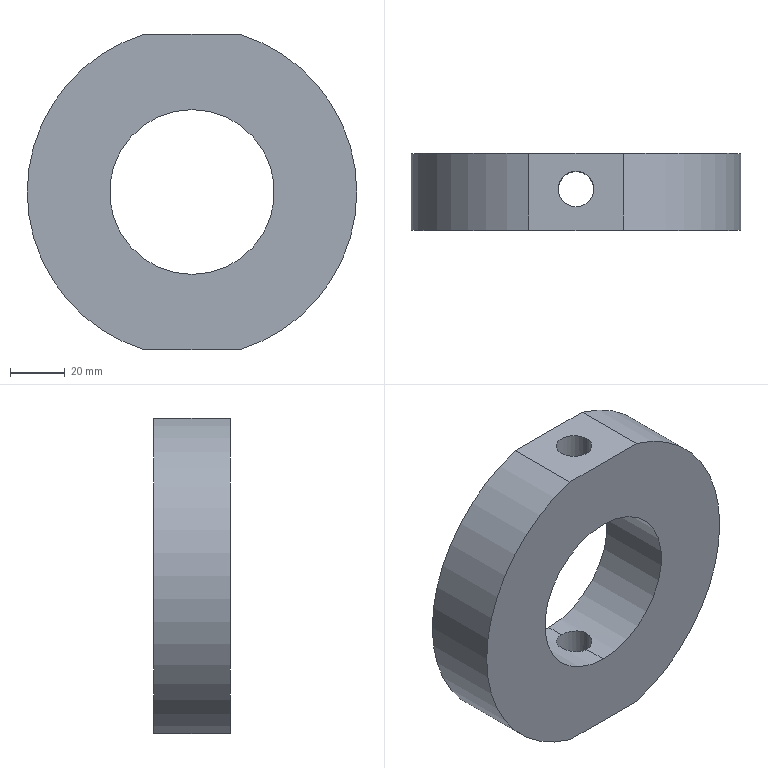Part | SolidWorks | features ICE 2, Extrusion 1 | 1 solid | 12 faces | box 120 x 28 x 115 mm | volume 226944 mm3 | cylinder 8 | plane 4 | commonest cylinder face diameters 13 x4 60 x2 120 x2
STEP:
#1=CARTESIAN_POINT('',(0.,-5.5,30.));
#2=VERTEX_POINT('',#1);
#3=CARTESIAN_POINT('',(-6.5,1.,29.287));
#4=VERTEX_POINT('',#3);
#5=CARTESIAN_POINT('',(0.,-5.5,30.));
#6=CARTESIAN_POINT('',(-0.4253,-5.5,30.));
#7=CARTESIAN_POINT('',(-0.8574,-5.457,29.991));
#8=CARTESIAN_POINT('',(-1.692,-5.29,29.955));
#9=CARTESIAN_POINT('',(-2.097,-5.167,29.929));
#10=CARTESIAN_POINT('',(-2.689,-4.922,29.88));
#11=CARTESIAN_POINT('',(-2.883,-4.829,29.862));
#12=CARTESIAN_POINT('',(-3.258,-4.628,29.823));
#13=CARTESIAN_POINT('',(-3.44,-4.519,29.803));
#14=CARTESIAN_POINT('',(-3.967,-4.167,29.739));
#15=CARTESIAN_POINT('',(-4.296,-3.896,29.692));
#16=CARTESIAN_POINT('',(-4.899,-3.293,29.599));
#17=CARTESIAN_POINT('',(-5.167,-2.966,29.553));
#18=CARTESIAN_POINT('',(-5.52,-2.439,29.488));
#19=CARTESIAN_POINT('',(-5.629,-2.257,29.467));
#20=CARTESIAN_POINT('',(-5.831,-1.88,29.428));
#21=CARTESIAN_POINT('',(-5.923,-1.686,29.41));
#22=CARTESIAN_POINT('',(-6.167,-1.097,29.36));
#23=CARTESIAN_POINT('',(-6.29,-0.692,29.333));
#24=CARTESIAN_POINT('',(-6.416,-0.06519,29.306));
#25=CARTESIAN_POINT('',(-6.448,0.1482,29.299));
#26=CARTESIAN_POINT('',(-6.49,0.5748,29.29));
#27=CARTESIAN_POINT('',(-6.5,0.7876,29.287));
#28=CARTESIAN_POINT('',(-6.5,1.,29.287));
#29=B_SPLINE_CURVE_WITH_KNOTS('',3,(#5,#6,#7,#8,#9,#10,#11,#12,#13,#14,#15,#16,#17,#18,#19,#20,#21,#22,#23,#24,#25,#26,#27,#28),.UNSPECIFIED.,.F.,.F.,(4,2,2,2,2,2,2,2,2,2,2,4),(0.01019,0.01147,0.01274,0.01338,0.01401,0.01529,0.01656,0.0172,0.01784,0.01911,0.01975,0.02038),.UNSPECIFIED.);
#30=EDGE_CURVE('',#2,#4,#29,.T.);
#31=ORIENTED_EDGE('',*,*,#30,.T.);
#32=CARTESIAN_POINT('',(-6.5,1.,57.5));
#33=VERTEX_POINT('',#32);
#34=CARTESIAN_POINT('',(-6.5,1.,-57.5));
#35=DIRECTION('',(0.,0.,1.));
#36=VECTOR('',#35,1000.);
#37=LINE('',#34,#36);
#38=EDGE_CURVE('',#4,#33,#37,.T.);
#39=ORIENTED_EDGE('',*,*,#38,.T.);
#40=CARTESIAN_POINT('',(6.5,1.,57.5));
#41=VERTEX_POINT('',#40);
#42=CARTESIAN_POINT('',(0.,1.,57.5));
#43=DIRECTION('',(0.,0.,1.));
#44=DIRECTION('',(1.,0.,0.));
#45=AXIS2_PLACEMENT_3D('',#42,#43,#44);
#46=CIRCLE('',#45,6.5);
#47=EDGE_CURVE('',#33,#41,#46,.T.);
#48=ORIENTED_EDGE('',*,*,#47,.T.);
#49=CARTESIAN_POINT('',(6.5,1.,29.287));
#50=VERTEX_POINT('',#49);
#51=CARTESIAN_POINT('',(6.5,1.,-57.5));
#52=DIRECTION('',(0.,0.,1.));
#53=VECTOR('',#52,1000.);
#54=LINE('',#51,#53);
#55=EDGE_CURVE('',#50,#41,#54,.T.);
#56=ORIENTED_EDGE('',*,*,#55,.F.);
#57=CARTESIAN_POINT('',(6.5,1.,29.287));
#58=CARTESIAN_POINT('',(6.5,0.569,29.287));
#59=CARTESIAN_POINT('',(6.458,0.1455,29.297));
#60=CARTESIAN_POINT('',(6.333,-0.479,29.324));
#61=CARTESIAN_POINT('',(6.281,-0.6854,29.335));
#62=CARTESIAN_POINT('',(6.157,-1.095,29.361));
#63=CARTESIAN_POINT('',(6.084,-1.298,29.377));
#64=CARTESIAN_POINT('',(5.839,-1.888,29.427));
#65=CARTESIAN_POINT('',(5.639,-2.26,29.466));
#66=CARTESIAN_POINT('',(5.167,-2.966,29.553));
#67=CARTESIAN_POINT('',(4.893,-3.299,29.6));
#68=CARTESIAN_POINT('',(4.295,-3.897,29.692));
#69=CARTESIAN_POINT('',(3.969,-4.166,29.738));
#70=CARTESIAN_POINT('',(3.258,-4.641,29.825));
#71=CARTESIAN_POINT('',(2.882,-4.842,29.864));
#72=CARTESIAN_POINT('',(2.295,-5.085,29.913));
#73=CARTESIAN_POINT('',(2.095,-5.157,29.927));
#74=CARTESIAN_POINT('',(1.688,-5.281,29.953));
#75=CARTESIAN_POINT('',(1.478,-5.333,29.964));
#76=CARTESIAN_POINT('',(0.8483,-5.459,29.991));
#77=CARTESIAN_POINT('',(0.4255,-5.5,30.));
#78=CARTESIAN_POINT('',(0.,-5.5,30.));
#79=B_SPLINE_CURVE_WITH_KNOTS('',3,(#57,#58,#59,#60,#61,#62,#63,#64,#65,#66,#67,#68,#69,#70,#71,#72,#73,#74,#75,#76,#77,#78),.UNSPECIFIED.,.F.,.F.,(4,2,2,2,2,2,2,2,2,2,4),(0.,0.001274,0.001911,0.002548,0.003823,0.005097,0.006371,0.007645,0.008282,0.00892,0.01019),.UNSPECIFIED.);
#80=EDGE_CURVE('',#50,#2,#79,.T.);
#81=ORIENTED_EDGE('',*,*,#80,.T.);
#82=EDGE_LOOP('',(#31,#39,#48,#56,#81));
#83=FACE_OUTER_BOUND('',#82,.T.);
#84=CARTESIAN_POINT('',(0.,1.,-57.5));
#85=DIRECTION('',(0.,0.,1.));
#86=DIRECTION('',(1.,0.,0.));
#87=AXIS2_PLACEMENT_3D('',#84,#85,#86);
#88=CYLINDRICAL_SURFACE('',#87,6.5);
#89=ADVANCED_FACE('',(#83),#88,.F.);
#90=CARTESIAN_POINT('',(-6.5,1.,-57.5));
#91=VERTEX_POINT('',#90);
#92=CARTESIAN_POINT('',(6.5,1.,-57.5));
#93=VERTEX_POINT('',#92);
#94=CARTESIAN_POINT('',(0.,1.,-57.5));
#95=DIRECTION('',(0.,0.,1.));
#96=DIRECTION('',(1.,0.,0.));
#97=AXIS2_PLACEMENT_3D('',#94,#95,#96);
#98=CIRCLE('',#97,6.5);
#99=EDGE_CURVE('',#91,#93,#98,.T.);
#100=ORIENTED_EDGE('',*,*,#99,.F.);
#101=CARTESIAN_POINT('',(-6.5,1.,-29.287));
#102=VERTEX_POINT('',#101);
#103=CARTESIAN_POINT('',(-6.5,1.,-57.5));
#104=DIRECTION('',(0.,0.,1.));
#105=VECTOR('',#104,1000.);
#106=LINE('',#103,#105);
#107=EDGE_CURVE('',#91,#102,#106,.T.);
#108=ORIENTED_EDGE('',*,*,#107,.T.);
#109=CARTESIAN_POINT('',(0.,-5.5,-30.));
#110=VERTEX_POINT('',#109);
#111=CARTESIAN_POINT('',(-6.5,1.,-29.287));
#112=CARTESIAN_POINT('',(-6.5,0.5747,-29.287));
#113=CARTESIAN_POINT('',(-6.457,0.1426,-29.297));
#114=CARTESIAN_POINT('',(-6.29,-0.6917,-29.333));
#115=CARTESIAN_POINT('',(-6.167,-1.097,-29.36));
#116=CARTESIAN_POINT('',(-5.922,-1.689,-29.41));
#117=CARTESIAN_POINT('',(-5.829,-1.883,-29.428));
#118=CARTESIAN_POINT('',(-5.628,-2.258,-29.467));
#119=CARTESIAN_POINT('',(-5.519,-2.44,-29.488));
#120=CARTESIAN_POINT('',(-5.167,-2.966,-29.553));
#121=CARTESIAN_POINT('',(-4.896,-3.296,-29.599));
#122=CARTESIAN_POINT('',(-4.293,-3.899,-29.693));
#123=CARTESIAN_POINT('',(-3.966,-4.167,-29.739));
#124=CARTESIAN_POINT('',(-3.439,-4.52,-29.803));
#125=CARTESIAN_POINT('',(-3.257,-4.629,-29.823));
#126=CARTESIAN_POINT('',(-2.88,-4.831,-29.862));
#127=CARTESIAN_POINT('',(-2.686,-4.923,-29.88));
#128=CARTESIAN_POINT('',(-2.097,-5.167,-29.929));
#129=CARTESIAN_POINT('',(-1.692,-5.29,-29.955));
#130=CARTESIAN_POINT('',(-1.065,-5.416,-29.982));
#131=CARTESIAN_POINT('',(-0.8518,-5.448,-29.989));
#132=CARTESIAN_POINT('',(-0.4252,-5.49,-29.998));
#133=CARTESIAN_POINT('',(-0.2124,-5.5,-30.));
#134=CARTESIAN_POINT('',(0.,-5.5,-30.));
#135=B_SPLINE_CURVE_WITH_KNOTS('',3,(#111,#112,#113,#114,#115,#116,#117,#118,#119,#120,#121,#122,#123,#124,#125,#126,#127,#128,#129,#130,#131,#132,#133,#134),.UNSPECIFIED.,.F.,.F.,(4,2,2,2,2,2,2,2,2,2,2,4),(0.01019,0.01147,0.01274,0.01338,0.01401,0.01529,0.01656,0.0172,0.01784,0.01911,0.01975,0.02038),.UNSPECIFIED.);
#136=EDGE_CURVE('',#102,#110,#135,.T.);
#137=ORIENTED_EDGE('',*,*,#136,.T.);
#138=CARTESIAN_POINT('',(6.5,1.,-29.287));
#139=VERTEX_POINT('',#138);
#140=CARTESIAN_POINT('',(0.,-5.5,-30.));
#141=CARTESIAN_POINT('',(0.4249,-5.5,-30.));
#142=CARTESIAN_POINT('',(0.8482,-5.459,-29.991));
#143=CARTESIAN_POINT('',(1.691,-5.291,-29.955));
#144=CARTESIAN_POINT('',(2.099,-5.166,-29.929));
#145=CARTESIAN_POINT('',(2.686,-4.923,-29.88));
#146=CARTESIAN_POINT('',(2.878,-4.832,-29.862));
#147=CARTESIAN_POINT('',(3.254,-4.631,-29.824));
#148=CARTESIAN_POINT('',(3.439,-4.52,-29.803));
#149=CARTESIAN_POINT('',(3.969,-4.165,-29.738));
#150=CARTESIAN_POINT('',(4.295,-3.897,-29.693));
#151=CARTESIAN_POINT('',(4.895,-3.298,-29.6));
#152=CARTESIAN_POINT('',(5.168,-2.965,-29.552));
#153=CARTESIAN_POINT('',(5.639,-2.261,-29.466));
#154=CARTESIAN_POINT('',(5.839,-1.888,-29.427));
#155=CARTESIAN_POINT('',(6.085,-1.296,-29.377));
#156=CARTESIAN_POINT('',(6.157,-1.094,-29.361));
#157=CARTESIAN_POINT('',(6.281,-0.6861,-29.335));
#158=CARTESIAN_POINT('',(6.384,-0.2744,-29.313));
#159=CARTESIAN_POINT('',(6.447,0.1457,-29.299));
#160=CARTESIAN_POINT('',(6.489,0.57,-29.29));
#161=CARTESIAN_POINT('',(6.5,0.7855,-29.287));
#162=CARTESIAN_POINT('',(6.5,1.,-29.287));
#163=B_SPLINE_CURVE_WITH_KNOTS('',3,(#140,#141,#142,#143,#144,#145,#146,#147,#148,#149,#150,#151,#152,#153,#154,#155,#156,#157,#158,#159,#160,#161,#162),.UNSPECIFIED.,.F.,.F.,(4,2,2,2,2,2,2,2,2,1,2,4),(0.02038,0.02166,0.02293,0.02357,0.0242,0.02548,0.02675,0.02803,0.02866,0.0293,0.02994,0.03057),.UNSPECIFIED.);
#164=EDGE_CURVE('',#110,#139,#163,.T.);
#165=ORIENTED_EDGE('',*,*,#164,.T.);
#166=CARTESIAN_POINT('',(6.5,1.,-57.5));
#167=DIRECTION('',(0.,0.,1.));
#168=VECTOR('',#167,1000.);
#169=LINE('',#166,#168);
#170=EDGE_CURVE('',#93,#139,#169,.T.);
#171=ORIENTED_EDGE('',*,*,#170,.F.);
#172=EDGE_LOOP('',(#100,#108,#137,#165,#171));
#173=FACE_OUTER_BOUND('',#172,.T.);
#174=CARTESIAN_POINT('',(0.,1.,-57.5));
#175=DIRECTION('',(0.,0.,1.));
#176=DIRECTION('',(1.,0.,0.));
#177=AXIS2_PLACEMENT_3D('',#174,#175,#176);
#178=CYLINDRICAL_SURFACE('',#177,6.5);
#179=ADVANCED_FACE('',(#173),#178,.F.);
#180=CARTESIAN_POINT('',(0.,14.,-30.));
#181=VERTEX_POINT('',#180);
#182=CARTESIAN_POINT('',(0.,14.,30.));
#183=VERTEX_POINT('',#182);
#184=CARTESIAN_POINT('',(0.,14.,0.));
#185=DIRECTION('',(0.,1.,0.));
#186=DIRECTION('',(0.,0.,1.));
#187=AXIS2_PLACEMENT_3D('',#184,#185,#186);
#188=CIRCLE('',#187,30.);
#189=EDGE_CURVE('',#181,#183,#188,.T.);
#190=ORIENTED_EDGE('',*,*,#189,.T.);
#191=CARTESIAN_POINT('',(0.,7.5,30.));
#192=VERTEX_POINT('',#191);
#193=CARTESIAN_POINT('',(0.,14.,30.));
#194=DIRECTION('',(0.,-1.,0.));
#195=VECTOR('',#194,1000.);
#196=LINE('',#193,#195);
#197=EDGE_CURVE('',#183,#192,#196,.T.);
#198=ORIENTED_EDGE('',*,*,#197,.T.);
#199=CARTESIAN_POINT('',(-6.5,1.,29.287));
#200=CARTESIAN_POINT('',(-6.5,1.425,29.287));
#201=CARTESIAN_POINT('',(-6.459,1.848,29.297));
#202=CARTESIAN_POINT('',(-6.291,2.691,29.333));
#203=CARTESIAN_POINT('',(-6.166,3.099,29.36));
#204=CARTESIAN_POINT('',(-5.923,3.686,29.41));
#205=CARTESIAN_POINT('',(-5.832,3.878,29.428));
#206=CARTESIAN_POINT('',(-5.631,4.254,29.467));
#207=CARTESIAN_POINT('',(-5.52,4.438,29.488));
#208=CARTESIAN_POINT('',(-5.165,4.968,29.553));
#209=CARTESIAN_POINT('',(-4.897,5.295,29.599));
#210=CARTESIAN_POINT('',(-4.298,5.894,29.692));
#211=CARTESIAN_POINT('',(-3.965,6.168,29.739));
#212=CARTESIAN_POINT('',(-3.261,6.638,29.824));
#213=CARTESIAN_POINT('',(-2.889,6.839,29.863));
#214=CARTESIAN_POINT('',(-2.296,7.085,29.913));
#215=CARTESIAN_POINT('',(-2.094,7.157,29.928));
#216=CARTESIAN_POINT('',(-1.686,7.281,29.953));
#217=CARTESIAN_POINT('',(-1.274,7.384,29.975));
#218=CARTESIAN_POINT('',(-0.8544,7.447,29.989));
#219=CARTESIAN_POINT('',(-0.43,7.489,29.998));
#220=CARTESIAN_POINT('',(-0.2145,7.5,30.));
#221=CARTESIAN_POINT('',(0.,7.5,30.));
#222=B_SPLINE_CURVE_WITH_KNOTS('',3,(#199,#200,#201,#202,#203,#204,#205,#206,#207,#208,#209,#210,#211,#212,#213,#214,#215,#216,#217,#218,#219,#220,#221),.UNSPECIFIED.,.F.,.F.,(4,2,2,2,2,2,2,2,2,1,2,4),(0.02038,0.02166,0.02293,0.02357,0.0242,0.02548,0.02675,0.02803,0.02866,0.0293,0.02994,0.03057),.UNSPECIFIED.);
#223=EDGE_CURVE('',#4,#192,#222,.T.);
#224=ORIENTED_EDGE('',*,*,#223,.F.);
#225=ORIENTED_EDGE('',*,*,#30,.F.);
#226=CARTESIAN_POINT('',(0.,-14.,30.));
#227=VERTEX_POINT('',#226);
#228=CARTESIAN_POINT('',(0.,14.,30.));
#229=DIRECTION('',(0.,-1.,0.));
#230=VECTOR('',#229,1000.);
#231=LINE('',#228,#230);
#232=EDGE_CURVE('',#2,#227,#231,.T.);
#233=ORIENTED_EDGE('',*,*,#232,.T.);
#234=CARTESIAN_POINT('',(0.,-14.,-30.));
#235=VERTEX_POINT('',#234);
#236=CARTESIAN_POINT('',(0.,-14.,0.));
#237=DIRECTION('',(0.,1.,0.));
#238=DIRECTION('',(0.,0.,1.));
#239=AXIS2_PLACEMENT_3D('',#236,#237,#238);
#240=CIRCLE('',#239,30.);
#241=EDGE_CURVE('',#235,#227,#240,.T.);
#242=ORIENTED_EDGE('',*,*,#241,.F.);
#243=CARTESIAN_POINT('',(0.,14.,-30.));
#244=DIRECTION('',(0.,-1.,0.));
#245=VECTOR('',#244,1000.);
#246=LINE('',#243,#245);
#247=EDGE_CURVE('',#110,#235,#246,.T.);
#248=ORIENTED_EDGE('',*,*,#247,.F.);
#249=ORIENTED_EDGE('',*,*,#136,.F.);
#250=CARTESIAN_POINT('',(0.,7.5,-30.));
#251=VERTEX_POINT('',#250);
#252=CARTESIAN_POINT('',(0.,7.5,-30.));
#253=CARTESIAN_POINT('',(-0.431,7.5,-30.));
#254=CARTESIAN_POINT('',(-0.8545,7.458,-29.991));
#255=CARTESIAN_POINT('',(-1.479,7.333,-29.964));
#256=CARTESIAN_POINT('',(-1.685,7.281,-29.953));
#257=CARTESIAN_POINT('',(-2.095,7.157,-29.927));
#258=CARTESIAN_POINT('',(-2.298,7.084,-29.913));
#259=CARTESIAN_POINT('',(-2.888,6.839,-29.863));
#260=CARTESIAN_POINT('',(-3.261,6.639,-29.824));
#261=CARTESIAN_POINT('',(-3.966,6.167,-29.739));
#262=CARTESIAN_POINT('',(-4.3,5.893,-29.692));
#263=CARTESIAN_POINT('',(-4.897,5.295,-29.599));
#264=CARTESIAN_POINT('',(-5.166,4.968,-29.553));
#265=CARTESIAN_POINT('',(-5.641,4.258,-29.466));
#266=CARTESIAN_POINT('',(-5.842,3.881,-29.426));
#267=CARTESIAN_POINT('',(-6.085,3.295,-29.377));
#268=CARTESIAN_POINT('',(-6.157,3.095,-29.362));
#269=CARTESIAN_POINT('',(-6.281,2.688,-29.335));
#270=CARTESIAN_POINT('',(-6.333,2.478,-29.324));
#271=CARTESIAN_POINT('',(-6.459,1.848,-29.297));
#272=CARTESIAN_POINT('',(-6.5,1.425,-29.287));
#273=CARTESIAN_POINT('',(-6.5,1.,-29.287));
#274=B_SPLINE_CURVE_WITH_KNOTS('',3,(#252,#253,#254,#255,#256,#257,#258,#259,#260,#261,#262,#263,#264,#265,#266,#267,#268,#269,#270,#271,#272,#273),.UNSPECIFIED.,.F.,.F.,(4,2,2,2,2,2,2,2,2,2,4),(0.,0.001274,0.001911,0.002548,0.003823,0.005097,0.006371,0.007645,0.008283,0.00892,0.01019),.UNSPECIFIED.);
#275=EDGE_CURVE('',#251,#102,#274,.T.);
#276=ORIENTED_EDGE('',*,*,#275,.F.);
#277=CARTESIAN_POINT('',(0.,14.,-30.));
#278=DIRECTION('',(0.,-1.,0.));
#279=VECTOR('',#278,1000.);
#280=LINE('',#277,#279);
#281=EDGE_CURVE('',#181,#251,#280,.T.);
#282=ORIENTED_EDGE('',*,*,#281,.F.);
#283=EDGE_LOOP('',(#190,#198,#224,#225,#233,#242,#248,#249,#276,#282));
#284=FACE_OUTER_BOUND('',#283,.T.);
#285=CARTESIAN_POINT('',(0.,14.,0.));
#286=DIRECTION('',(0.,-1.,0.));
#287=DIRECTION('',(0.,0.,-1.));
#288=AXIS2_PLACEMENT_3D('',#285,#286,#287);
#289=CYLINDRICAL_SURFACE('',#288,30.);
#290=ADVANCED_FACE('',(#284),#289,.F.);
#291=ORIENTED_EDGE('',*,*,#189,.F.);
#292=CARTESIAN_POINT('',(0.,14.,0.));
#293=DIRECTION('',(0.,1.,0.));
#294=DIRECTION('',(0.,0.,1.));
#295=AXIS2_PLACEMENT_3D('',#292,#293,#294);
#296=CIRCLE('',#295,30.);
#297=EDGE_CURVE('',#183,#181,#296,.T.);
#298=ORIENTED_EDGE('',*,*,#297,.F.);
#299=EDGE_LOOP('',(#291,#298));
#300=FACE_BOUND('',#299,.T.);
#301=CARTESIAN_POINT('',(17.139,14.,57.5));
#302=VERTEX_POINT('',#301);
#303=CARTESIAN_POINT('',(17.139,14.,-57.5));
#304=VERTEX_POINT('',#303);
#305=CARTESIAN_POINT('',(0.,14.,0.));
#306=DIRECTION('',(0.,1.,0.));
#307=DIRECTION('',(0.,0.,1.));
#308=AXIS2_PLACEMENT_3D('',#305,#306,#307);
#309=CIRCLE('',#308,60.);
#310=EDGE_CURVE('',#302,#304,#309,.T.);
#311=ORIENTED_EDGE('',*,*,#310,.T.);
#312=CARTESIAN_POINT('',(-17.139,14.,-57.5));
#313=VERTEX_POINT('',#312);
#314=CARTESIAN_POINT('',(-80.,14.,-57.5));
#315=DIRECTION('',(-1.,0.,0.));
#316=VECTOR('',#315,1000.);
#317=LINE('',#314,#316);
#318=EDGE_CURVE('',#304,#313,#317,.T.);
#319=ORIENTED_EDGE('',*,*,#318,.T.);
#320=CARTESIAN_POINT('',(-17.139,14.,57.5));
#321=VERTEX_POINT('',#320);
#322=CARTESIAN_POINT('',(0.,14.,0.));
#323=DIRECTION('',(0.,1.,0.));
#324=DIRECTION('',(0.,0.,1.));
#325=AXIS2_PLACEMENT_3D('',#322,#323,#324);
#326=CIRCLE('',#325,60.);
#327=EDGE_CURVE('',#313,#321,#326,.T.);
#328=ORIENTED_EDGE('',*,*,#327,.T.);
#329=CARTESIAN_POINT('',(-80.,14.,57.5));
#330=DIRECTION('',(1.,0.,0.));
#331=VECTOR('',#330,1000.);
#332=LINE('',#329,#331);
#333=EDGE_CURVE('',#321,#302,#332,.T.);
#334=ORIENTED_EDGE('',*,*,#333,.T.);
#335=EDGE_LOOP('',(#311,#319,#328,#334));
#336=FACE_OUTER_BOUND('',#335,.T.);
#337=CARTESIAN_POINT('',(0.,14.,0.));
#338=DIRECTION('',(0.,1.,0.));
#339=DIRECTION('',(0.,0.,1.));
#340=AXIS2_PLACEMENT_3D('',#337,#338,#339);
#341=PLANE('',#340);
#342=ADVANCED_FACE('',(#300,#336),#341,.T.);
#343=ORIENTED_EDGE('',*,*,#241,.T.);
#344=CARTESIAN_POINT('',(0.,-14.,0.));
#345=DIRECTION('',(0.,1.,0.));
#346=DIRECTION('',(0.,0.,1.));
#347=AXIS2_PLACEMENT_3D('',#344,#345,#346);
#348=CIRCLE('',#347,30.);
#349=EDGE_CURVE('',#227,#235,#348,.T.);
#350=ORIENTED_EDGE('',*,*,#349,.T.);
#351=EDGE_LOOP('',(#343,#350));
#352=FACE_BOUND('',#351,.T.);
#353=CARTESIAN_POINT('',(17.139,-14.,-57.5));
#354=VERTEX_POINT('',#353);
#355=CARTESIAN_POINT('',(-17.139,-14.,-57.5));
#356=VERTEX_POINT('',#355);
#357=CARTESIAN_POINT('',(-80.,-14.,-57.5));
#358=DIRECTION('',(-1.,0.,0.));
#359=VECTOR('',#358,1000.);
#360=LINE('',#357,#359);
#361=EDGE_CURVE('',#354,#356,#360,.T.);
#362=ORIENTED_EDGE('',*,*,#361,.F.);
#363=CARTESIAN_POINT('',(17.139,-14.,57.5));
#364=VERTEX_POINT('',#363);
#365=CARTESIAN_POINT('',(0.,-14.,0.));
#366=DIRECTION('',(0.,1.,0.));
#367=DIRECTION('',(0.,0.,1.));
#368=AXIS2_PLACEMENT_3D('',#365,#366,#367);
#369=CIRCLE('',#368,60.);
#370=EDGE_CURVE('',#364,#354,#369,.T.);
#371=ORIENTED_EDGE('',*,*,#370,.F.);
#372=CARTESIAN_POINT('',(-17.139,-14.,57.5));
#373=VERTEX_POINT('',#372);
#374=CARTESIAN_POINT('',(-80.,-14.,57.5));
#375=DIRECTION('',(1.,0.,0.));
#376=VECTOR('',#375,1000.);
#377=LINE('',#374,#376);
#378=EDGE_CURVE('',#373,#364,#377,.T.);
#379=ORIENTED_EDGE('',*,*,#378,.F.);
#380=CARTESIAN_POINT('',(0.,-14.,0.));
#381=DIRECTION('',(0.,1.,0.));
#382=DIRECTION('',(0.,0.,1.));
#383=AXIS2_PLACEMENT_3D('',#380,#381,#382);
#384=CIRCLE('',#383,60.);
#385=EDGE_CURVE('',#356,#373,#384,.T.);
#386=ORIENTED_EDGE('',*,*,#385,.F.);
#387=EDGE_LOOP('',(#362,#371,#379,#386));
#388=FACE_OUTER_BOUND('',#387,.T.);
#389=CARTESIAN_POINT('',(0.,-14.,0.));
#390=DIRECTION('',(0.,1.,0.));
#391=DIRECTION('',(0.,0.,1.));
#392=AXIS2_PLACEMENT_3D('',#389,#390,#391);
#393=PLANE('',#392);
#394=ADVANCED_FACE('',(#352,#388),#393,.F.);
#395=CARTESIAN_POINT('',(17.139,14.,-57.5));
#396=DIRECTION('',(0.,-1.,0.));
#397=VECTOR('',#396,1000.);
#398=LINE('',#395,#397);
#399=EDGE_CURVE('',#304,#354,#398,.T.);
#400=ORIENTED_EDGE('',*,*,#399,.F.);
#401=ORIENTED_EDGE('',*,*,#310,.F.);
#402=CARTESIAN_POINT('',(17.139,14.,57.5));
#403=DIRECTION('',(0.,1.,0.));
#404=VECTOR('',#403,1000.);
#405=LINE('',#402,#404);
#406=EDGE_CURVE('',#364,#302,#405,.T.);
#407=ORIENTED_EDGE('',*,*,#406,.F.);
#408=ORIENTED_EDGE('',*,*,#370,.T.);
#409=EDGE_LOOP('',(#400,#401,#407,#408));
#410=FACE_OUTER_BOUND('',#409,.T.);
#411=CARTESIAN_POINT('',(0.,14.,0.));
#412=DIRECTION('',(0.,-1.,0.));
#413=DIRECTION('',(0.,0.,-1.));
#414=AXIS2_PLACEMENT_3D('',#411,#412,#413);
#415=CYLINDRICAL_SURFACE('',#414,60.);
#416=ADVANCED_FACE('',(#410),#415,.T.);
#417=CARTESIAN_POINT('',(-17.139,14.,-57.5));
#418=DIRECTION('',(0.,1.,0.));
#419=VECTOR('',#418,1000.);
#420=LINE('',#417,#419);
#421=EDGE_CURVE('',#356,#313,#420,.T.);
#422=ORIENTED_EDGE('',*,*,#421,.F.);
#423=ORIENTED_EDGE('',*,*,#385,.T.);
#424=CARTESIAN_POINT('',(-17.139,14.,57.5));
#425=DIRECTION('',(0.,-1.,0.));
#426=VECTOR('',#425,1000.);
#427=LINE('',#424,#426);
#428=EDGE_CURVE('',#321,#373,#427,.T.);
#429=ORIENTED_EDGE('',*,*,#428,.F.);
#430=ORIENTED_EDGE('',*,*,#327,.F.);
#431=EDGE_LOOP('',(#422,#423,#429,#430));
#432=FACE_OUTER_BOUND('',#431,.T.);
#433=CARTESIAN_POINT('',(0.,14.,0.));
#434=DIRECTION('',(0.,-1.,0.));
#435=DIRECTION('',(0.,0.,-1.));
#436=AXIS2_PLACEMENT_3D('',#433,#434,#435);
#437=CYLINDRICAL_SURFACE('',#436,60.);
#438=ADVANCED_FACE('',(#432),#437,.T.);
#439=ORIENTED_EDGE('',*,*,#197,.F.);
#440=ORIENTED_EDGE('',*,*,#297,.T.);
#441=ORIENTED_EDGE('',*,*,#281,.T.);
#442=CARTESIAN_POINT('',(6.5,1.,-29.287));
#443=CARTESIAN_POINT('',(6.5,1.429,-29.287));
#444=CARTESIAN_POINT('',(6.458,1.852,-29.297));
#445=CARTESIAN_POINT('',(6.292,2.685,-29.333));
#446=CARTESIAN_POINT('',(6.166,3.099,-29.36));
#447=CARTESIAN_POINT('',(5.841,3.884,-29.426));
#448=CARTESIAN_POINT('',(5.641,4.257,-29.466));
#449=CARTESIAN_POINT('',(5.287,4.787,-29.531));
#450=CARTESIAN_POINT('',(5.159,4.96,-29.553));
#451=CARTESIAN_POINT('',(4.889,5.288,-29.599));
#452=CARTESIAN_POINT('',(4.747,5.445,-29.622));
#453=CARTESIAN_POINT('',(4.3,5.893,-29.692));
#454=CARTESIAN_POINT('',(3.972,6.163,-29.738));
#455=CARTESIAN_POINT('',(3.261,6.639,-29.824));
#456=CARTESIAN_POINT('',(2.888,6.838,-29.863));
#457=CARTESIAN_POINT('',(2.302,7.082,-29.912));
#458=CARTESIAN_POINT('',(2.102,7.154,-29.927));
#459=CARTESIAN_POINT('',(1.693,7.279,-29.953));
#460=CARTESIAN_POINT('',(1.484,7.332,-29.964));
#461=CARTESIAN_POINT('',(0.8554,7.458,-29.991));
#462=CARTESIAN_POINT('',(0.4306,7.5,-30.));
#463=CARTESIAN_POINT('',(0.,7.5,-30.));
#464=B_SPLINE_CURVE_WITH_KNOTS('',3,(#442,#443,#444,#445,#446,#447,#448,#449,#450,#451,#452,#453,#454,#455,#456,#457,#458,#459,#460,#461,#462,#463),.UNSPECIFIED.,.F.,.F.,(4,2,2,2,2,2,2,2,2,2,4),(0.03057,0.03185,0.03312,0.03439,0.03503,0.03567,0.03694,0.03821,0.03885,0.03949,0.04076),.UNSPECIFIED.);
#465=EDGE_CURVE('',#139,#251,#464,.T.);
#466=ORIENTED_EDGE('',*,*,#465,.F.);
#467=ORIENTED_EDGE('',*,*,#164,.F.);
#468=ORIENTED_EDGE('',*,*,#247,.T.);
#469=ORIENTED_EDGE('',*,*,#349,.F.);
#470=ORIENTED_EDGE('',*,*,#232,.F.);
#471=ORIENTED_EDGE('',*,*,#80,.F.);
#472=CARTESIAN_POINT('',(0.,7.5,30.));
#473=CARTESIAN_POINT('',(0.4288,7.5,30.));
#474=CARTESIAN_POINT('',(0.8515,7.458,29.991));
#475=CARTESIAN_POINT('',(1.685,7.292,29.956));
#476=CARTESIAN_POINT('',(2.099,7.166,29.929));
#477=CARTESIAN_POINT('',(2.884,6.841,29.864));
#478=CARTESIAN_POINT('',(3.257,6.641,29.825));
#479=CARTESIAN_POINT('',(3.788,6.287,29.76));
#480=CARTESIAN_POINT('',(3.96,6.159,29.738));
#481=CARTESIAN_POINT('',(4.289,5.889,29.692));
#482=CARTESIAN_POINT('',(4.445,5.747,29.669));
#483=CARTESIAN_POINT('',(4.893,5.3,29.6));
#484=CARTESIAN_POINT('',(5.163,4.972,29.553));
#485=CARTESIAN_POINT('',(5.639,4.261,29.466));
#486=CARTESIAN_POINT('',(5.839,3.888,29.427));
#487=CARTESIAN_POINT('',(6.082,3.302,29.377));
#488=CARTESIAN_POINT('',(6.154,3.102,29.362));
#489=CARTESIAN_POINT('',(6.279,2.693,29.336));
#490=CARTESIAN_POINT('',(6.332,2.484,29.324));
#491=CARTESIAN_POINT('',(6.458,1.855,29.297));
#492=CARTESIAN_POINT('',(6.5,1.431,29.287));
#493=CARTESIAN_POINT('',(6.5,1.,29.287));
#494=B_SPLINE_CURVE_WITH_KNOTS('',3,(#472,#473,#474,#475,#476,#477,#478,#479,#480,#481,#482,#483,#484,#485,#486,#487,#488,#489,#490,#491,#492,#493),.UNSPECIFIED.,.F.,.F.,(4,2,2,2,2,2,2,2,2,2,4),(0.03057,0.03185,0.03312,0.03439,0.03503,0.03567,0.03694,0.03821,0.03885,0.03949,0.04076),.UNSPECIFIED.);
#495=EDGE_CURVE('',#192,#50,#494,.T.);
#496=ORIENTED_EDGE('',*,*,#495,.F.);
#497=EDGE_LOOP('',(#439,#440,#441,#466,#467,#468,#469,#470,#471,#496));
#498=FACE_OUTER_BOUND('',#497,.T.);
#499=CARTESIAN_POINT('',(0.,14.,0.));
#500=DIRECTION('',(0.,-1.,0.));
#501=DIRECTION('',(0.,0.,-1.));
#502=AXIS2_PLACEMENT_3D('',#499,#500,#501);
#503=CYLINDRICAL_SURFACE('',#502,30.);
#504=ADVANCED_FACE('',(#498),#503,.F.);
#505=CARTESIAN_POINT('',(0.,1.,57.5));
#506=DIRECTION('',(0.,0.,1.));
#507=DIRECTION('',(1.,0.,0.));
#508=AXIS2_PLACEMENT_3D('',#505,#506,#507);
#509=CIRCLE('',#508,6.5);
#510=EDGE_CURVE('',#41,#33,#509,.T.);
#511=ORIENTED_EDGE('',*,*,#510,.F.);
#512=ORIENTED_EDGE('',*,*,#47,.F.);
#513=EDGE_LOOP('',(#511,#512));
#514=FACE_BOUND('',#513,.T.);
#515=ORIENTED_EDGE('',*,*,#428,.T.);
#516=ORIENTED_EDGE('',*,*,#378,.T.);
#517=ORIENTED_EDGE('',*,*,#406,.T.);
#518=ORIENTED_EDGE('',*,*,#333,.F.);
#519=EDGE_LOOP('',(#515,#516,#517,#518));
#520=FACE_OUTER_BOUND('',#519,.T.);
#521=CARTESIAN_POINT('',(-80.,-14.,57.5));
#522=DIRECTION('',(0.,0.,1.));
#523=DIRECTION('',(1.,0.,0.));
#524=AXIS2_PLACEMENT_3D('',#521,#522,#523);
#525=PLANE('',#524);
#526=ADVANCED_FACE('',(#514,#520),#525,.T.);
#527=CARTESIAN_POINT('',(0.,1.,-57.5));
#528=DIRECTION('',(0.,0.,1.));
#529=DIRECTION('',(1.,0.,0.));
#530=AXIS2_PLACEMENT_3D('',#527,#528,#529);
#531=CIRCLE('',#530,6.5);
#532=EDGE_CURVE('',#93,#91,#531,.T.);
#533=ORIENTED_EDGE('',*,*,#532,.T.);
#534=ORIENTED_EDGE('',*,*,#99,.T.);
#535=EDGE_LOOP('',(#533,#534));
#536=FACE_BOUND('',#535,.T.);
#537=ORIENTED_EDGE('',*,*,#399,.T.);
#538=ORIENTED_EDGE('',*,*,#361,.T.);
#539=ORIENTED_EDGE('',*,*,#421,.T.);
#540=ORIENTED_EDGE('',*,*,#318,.F.);
#541=EDGE_LOOP('',(#537,#538,#539,#540));
#542=FACE_OUTER_BOUND('',#541,.T.);
#543=CARTESIAN_POINT('',(-80.,-14.,-57.5));
#544=DIRECTION('',(0.,0.,-1.));
#545=DIRECTION('',(-1.,0.,0.));
#546=AXIS2_PLACEMENT_3D('',#543,#544,#545);
#547=PLANE('',#546);
#548=ADVANCED_FACE('',(#536,#542),#547,.T.);
#549=ORIENTED_EDGE('',*,*,#107,.F.);
#550=ORIENTED_EDGE('',*,*,#532,.F.);
#551=ORIENTED_EDGE('',*,*,#170,.T.);
#552=ORIENTED_EDGE('',*,*,#465,.T.);
#553=ORIENTED_EDGE('',*,*,#275,.T.);
#554=EDGE_LOOP('',(#549,#550,#551,#552,#553));
#555=FACE_OUTER_BOUND('',#554,.T.);
#556=CARTESIAN_POINT('',(0.,1.,-57.5));
#557=DIRECTION('',(0.,0.,1.));
#558=DIRECTION('',(1.,0.,0.));
#559=AXIS2_PLACEMENT_3D('',#556,#557,#558);
#560=CYLINDRICAL_SURFACE('',#559,6.5);
#561=ADVANCED_FACE('',(#555),#560,.F.);
#562=ORIENTED_EDGE('',*,*,#38,.F.);
#563=ORIENTED_EDGE('',*,*,#223,.T.);
#564=ORIENTED_EDGE('',*,*,#495,.T.);
#565=ORIENTED_EDGE('',*,*,#55,.T.);
#566=ORIENTED_EDGE('',*,*,#510,.T.);
#567=EDGE_LOOP('',(#562,#563,#564,#565,#566));
#568=FACE_OUTER_BOUND('',#567,.T.);
#569=CARTESIAN_POINT('',(0.,1.,-57.5));
#570=DIRECTION('',(0.,0.,1.));
#571=DIRECTION('',(1.,0.,0.));
#572=AXIS2_PLACEMENT_3D('',#569,#570,#571);
#573=CYLINDRICAL_SURFACE('',#572,6.5);
#574=ADVANCED_FACE('',(#568),#573,.F.);
#575=CLOSED_SHELL('',(#89,#179,#290,#342,#394,#416,#438,#504,#526,#548,#561,#574));
#576=MANIFOLD_SOLID_BREP('',#575);
#577=CARTESIAN_POINT('',(0.,0.,0.));
#578=DIRECTION('',(0.,0.,1.));
#579=DIRECTION('',(1.,0.,0.));
#580=AXIS2_PLACEMENT_3D('',#577,#578,#579);
#581=(LENGTH_UNIT()NAMED_UNIT(*)SI_UNIT(.MILLI.,.METRE.));
#582=UNCERTAINTY_MEASURE_WITH_UNIT(LENGTH_MEASURE(0.00001),#581,'','');
#583=(NAMED_UNIT(*)PLANE_ANGLE_UNIT()SI_UNIT($,.RADIAN.));
#584=(NAMED_UNIT(*)SI_UNIT($,.STERADIAN.)SOLID_ANGLE_UNIT());
#585=(GEOMETRIC_REPRESENTATION_CONTEXT(3)GLOBAL_UNCERTAINTY_ASSIGNED_CONTEXT((#582))GLOBAL_UNIT_ASSIGNED_CONTEXT((#581,#583,#584))REPRESENTATION_CONTEXT('',''));
#586=ADVANCED_BREP_SHAPE_REPRESENTATION('',(#576,#580),#585);